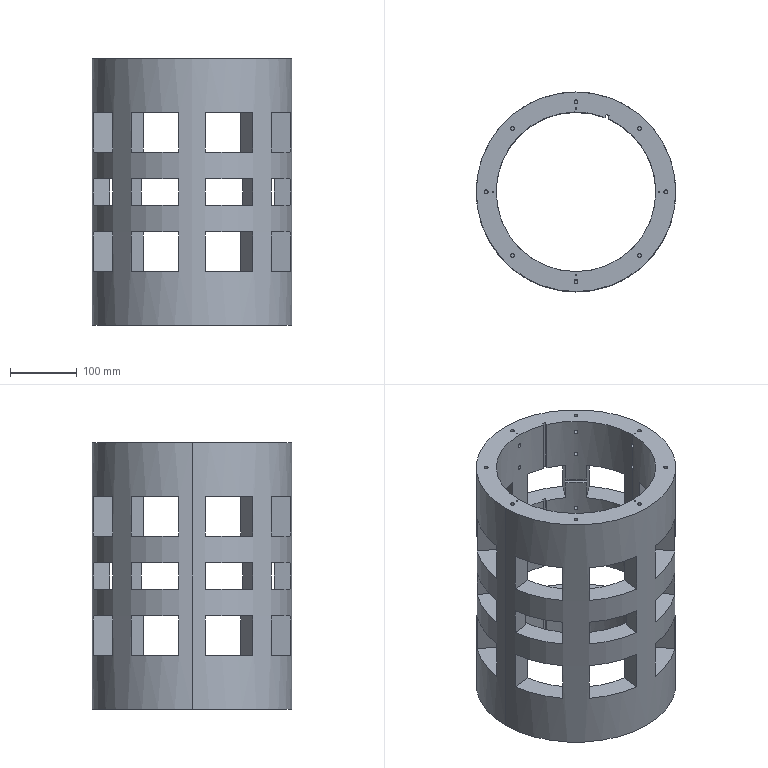Part | SolidWorks | features ICE 11, CirPattern 2, MirrorPattern 2, Extrusion 1, RevCut 1 | 1 solid | 281 faces | box 300 x 300 x 400 mm | volume 7301837 mm3 | cylinder 165 | plane 116 | commonest cylinder face diameters 6 x130 2 x16 250 x11 240 x6 300 x2